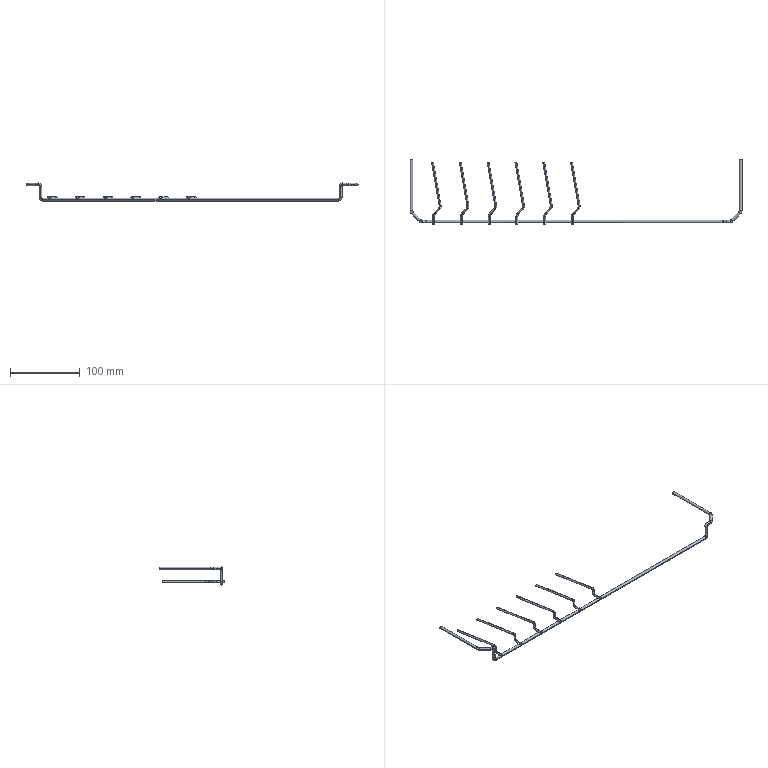Part | STEP file | ZXW722-L-178_XIAGEJIA_19_1_2_3_ | 1 solid | 108 faces | box 477.6 x 93 x 25.9 mm | volume 11494 mm3 | cylinder 54 | torus 40 | plane 14 | commonest cylinder face diameters 2.8 x36 3.9 x18